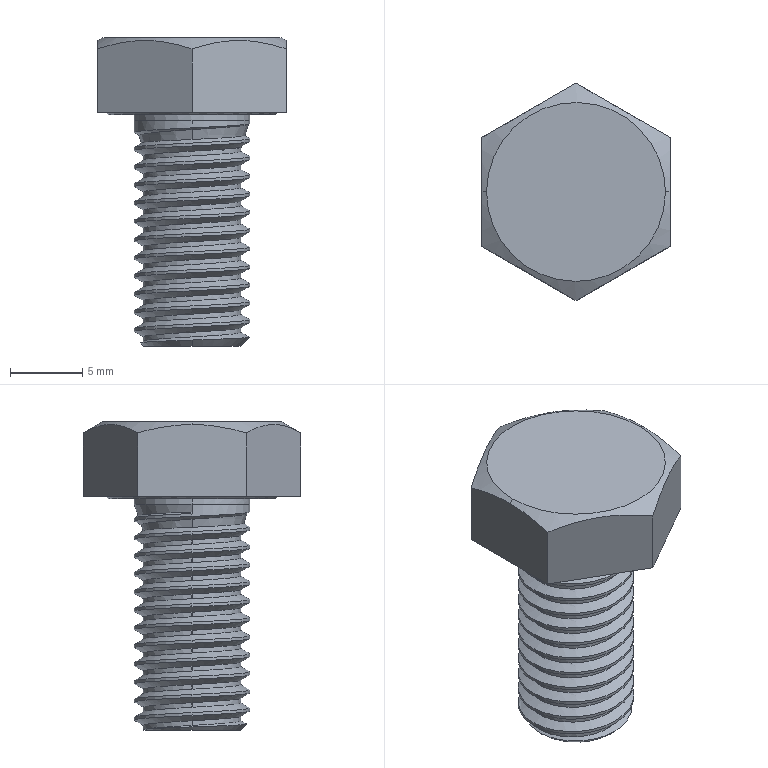Part | SolidWorks | features BaseBody 2 | 2 solids | 86 faces | box 13 x 15.011 x 21.3 mm | volume 1447 mm3 | cylinder 54 | cone 16 | plane 12 | spline 4 | commonest cylinder face diameters 8 x27 6.75 x23 6.645 x2 6.647 x2